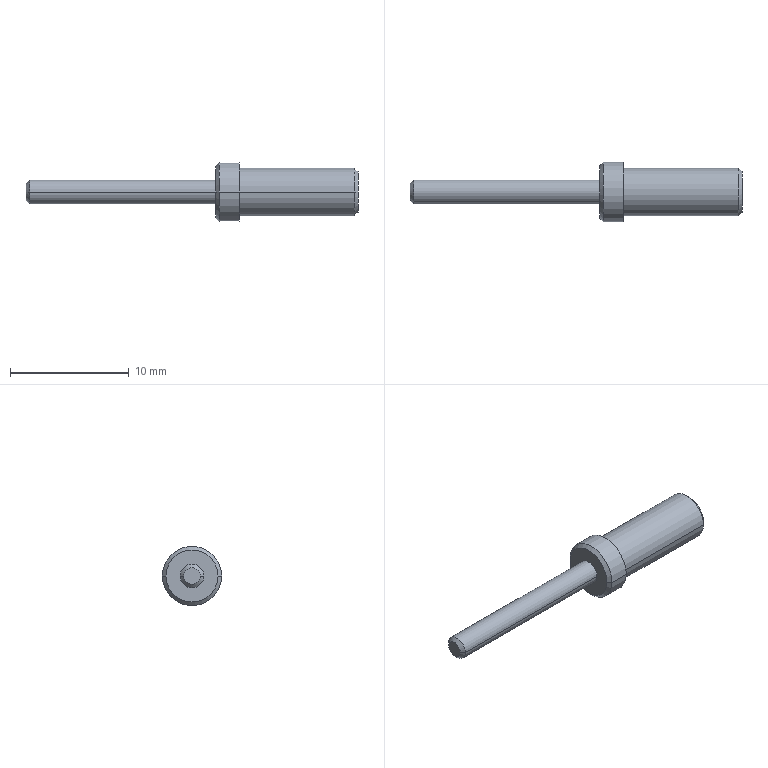Part | NX | 1 solid | 16 faces | box 28 x 5 x 5 mm | volume 213.729 mm3 | cylinder 6 | cone 6 | plane 4 | commonest cylinder face diameters 2 x2 4 x2 5 x2
STEP:
#1=CARTESIAN_POINT('',(2216.,157.,-96.));
#2=VERTEX_POINT('',#1);
#3=CARTESIAN_POINT('',(2216.,153.,-96.));
#4=VERTEX_POINT('',#3);
#5=CARTESIAN_POINT('',(2216.,155.,-96.));
#6=DIRECTION('',(1.,0.,0.));
#7=DIRECTION('',(0.,1.,0.));
#8=AXIS2_PLACEMENT_3D('',#5,#6,#7);
#9=CIRCLE('',#8,2.);
#10=EDGE_CURVE('',#2,#4,#9,.T.);
#11=ORIENTED_EDGE('',*,*,#10,.T.);
#12=CARTESIAN_POINT('',(2225.7,153.,-96.));
#13=VERTEX_POINT('',#12);
#14=CARTESIAN_POINT('',(2216.,153.,-96.));
#15=DIRECTION('',(1.,0.,0.));
#16=VECTOR('',#15,1000.);
#17=LINE('',#14,#16);
#18=EDGE_CURVE('',#4,#13,#17,.T.);
#19=ORIENTED_EDGE('',*,*,#18,.T.);
#20=CARTESIAN_POINT('',(2225.7,157.,-96.));
#21=VERTEX_POINT('',#20);
#22=CARTESIAN_POINT('',(2225.7,155.,-96.));
#23=DIRECTION('',(1.,0.,0.));
#24=DIRECTION('',(0.,1.,0.));
#25=AXIS2_PLACEMENT_3D('',#22,#23,#24);
#26=CIRCLE('',#25,2.);
#27=EDGE_CURVE('',#21,#13,#26,.T.);
#28=ORIENTED_EDGE('',*,*,#27,.F.);
#29=CARTESIAN_POINT('',(2216.,157.,-96.));
#30=DIRECTION('',(1.,0.,0.));
#31=VECTOR('',#30,1000.);
#32=LINE('',#29,#31);
#33=EDGE_CURVE('',#2,#21,#32,.T.);
#34=ORIENTED_EDGE('',*,*,#33,.F.);
#35=EDGE_LOOP('',(#11,#19,#28,#34));
#36=FACE_BOUND('',#35,.T.);
#37=CARTESIAN_POINT('',(2216.,155.,-96.));
#38=DIRECTION('',(1.,0.,0.));
#39=DIRECTION('',(0.,1.,0.));
#40=AXIS2_PLACEMENT_3D('',#37,#38,#39);
#41=CYLINDRICAL_SURFACE('',#40,2.);
#42=ADVANCED_FACE('',(#36),#41,.T.);
#43=CARTESIAN_POINT('',(2216.,152.5,-96.));
#44=VERTEX_POINT('',#43);
#45=CARTESIAN_POINT('',(2216.,157.5,-96.));
#46=VERTEX_POINT('',#45);
#47=CARTESIAN_POINT('',(2216.,155.,-96.));
#48=DIRECTION('',(1.,0.,0.));
#49=DIRECTION('',(0.,1.,0.));
#50=AXIS2_PLACEMENT_3D('',#47,#48,#49);
#51=CIRCLE('',#50,2.5);
#52=EDGE_CURVE('',#44,#46,#51,.T.);
#53=ORIENTED_EDGE('',*,*,#52,.T.);
#54=CARTESIAN_POINT('',(2216.,155.,-96.));
#55=DIRECTION('',(1.,0.,0.));
#56=DIRECTION('',(0.,1.,0.));
#57=AXIS2_PLACEMENT_3D('',#54,#55,#56);
#58=CIRCLE('',#57,2.5);
#59=EDGE_CURVE('',#46,#44,#58,.T.);
#60=ORIENTED_EDGE('',*,*,#59,.T.);
#61=EDGE_LOOP('',(#53,#60));
#62=FACE_BOUND('',#61,.T.);
#63=ORIENTED_EDGE('',*,*,#10,.F.);
#64=CARTESIAN_POINT('',(2216.,155.,-96.));
#65=DIRECTION('',(1.,0.,0.));
#66=DIRECTION('',(0.,1.,0.));
#67=AXIS2_PLACEMENT_3D('',#64,#65,#66);
#68=CIRCLE('',#67,2.);
#69=EDGE_CURVE('',#4,#2,#68,.T.);
#70=ORIENTED_EDGE('',*,*,#69,.F.);
#71=EDGE_LOOP('',(#63,#70));
#72=FACE_BOUND('',#71,.T.);
#73=CARTESIAN_POINT('',(2216.,153.76,-100.896));
#74=DIRECTION('',(1.,0.,0.));
#75=DIRECTION('',(0.,1.,0.));
#76=AXIS2_PLACEMENT_3D('',#73,#74,#75);
#77=PLANE('',#76);
#78=ADVANCED_FACE('',(#62,#72),#77,.T.);
#79=CARTESIAN_POINT('',(2214.3,152.5,-96.));
#80=VERTEX_POINT('',#79);
#81=CARTESIAN_POINT('',(2214.3,157.5,-96.));
#82=VERTEX_POINT('',#81);
#83=CARTESIAN_POINT('',(2214.3,155.,-96.));
#84=DIRECTION('',(1.,0.,0.));
#85=DIRECTION('',(0.,1.,0.));
#86=AXIS2_PLACEMENT_3D('',#83,#84,#85);
#87=CIRCLE('',#86,2.5);
#88=EDGE_CURVE('',#80,#82,#87,.T.);
#89=ORIENTED_EDGE('',*,*,#88,.T.);
#90=CARTESIAN_POINT('',(2216.,157.5,-96.));
#91=DIRECTION('',(1.,0.,0.));
#92=VECTOR('',#91,1000.);
#93=LINE('',#90,#92);
#94=EDGE_CURVE('',#82,#46,#93,.T.);
#95=ORIENTED_EDGE('',*,*,#94,.T.);
#96=ORIENTED_EDGE('',*,*,#52,.F.);
#97=CARTESIAN_POINT('',(2216.,152.5,-96.));
#98=DIRECTION('',(1.,0.,0.));
#99=VECTOR('',#98,1000.);
#100=LINE('',#97,#99);
#101=EDGE_CURVE('',#80,#44,#100,.T.);
#102=ORIENTED_EDGE('',*,*,#101,.F.);
#103=EDGE_LOOP('',(#89,#95,#96,#102));
#104=FACE_BOUND('',#103,.T.);
#105=CARTESIAN_POINT('',(2216.,155.,-96.));
#106=DIRECTION('',(1.,0.,0.));
#107=DIRECTION('',(0.,1.,0.));
#108=AXIS2_PLACEMENT_3D('',#105,#106,#107);
#109=CYLINDRICAL_SURFACE('',#108,2.5);
#110=ADVANCED_FACE('',(#104),#109,.T.);
#111=CARTESIAN_POINT('',(2214.,157.2,-96.));
#112=VERTEX_POINT('',#111);
#113=CARTESIAN_POINT('',(2214.,152.8,-96.));
#114=VERTEX_POINT('',#113);
#115=CARTESIAN_POINT('',(2214.,155.,-96.));
#116=DIRECTION('',(1.,0.,0.));
#117=DIRECTION('',(0.,1.,0.));
#118=AXIS2_PLACEMENT_3D('',#115,#116,#117);
#119=CIRCLE('',#118,2.2);
#120=EDGE_CURVE('',#112,#114,#119,.T.);
#121=ORIENTED_EDGE('',*,*,#120,.F.);
#122=CARTESIAN_POINT('',(2214.,155.,-96.));
#123=DIRECTION('',(1.,0.,0.));
#124=DIRECTION('',(0.,1.,0.));
#125=AXIS2_PLACEMENT_3D('',#122,#123,#124);
#126=CIRCLE('',#125,2.2);
#127=EDGE_CURVE('',#114,#112,#126,.T.);
#128=ORIENTED_EDGE('',*,*,#127,.F.);
#129=EDGE_LOOP('',(#121,#128));
#130=FACE_BOUND('',#129,.T.);
#131=CARTESIAN_POINT('',(2214.,156.,-96.));
#132=VERTEX_POINT('',#131);
#133=CARTESIAN_POINT('',(2214.,154.,-96.));
#134=VERTEX_POINT('',#133);
#135=CARTESIAN_POINT('',(2214.,155.,-96.));
#136=DIRECTION('',(-1.,0.,0.));
#137=DIRECTION('',(0.,-1.,0.));
#138=AXIS2_PLACEMENT_3D('',#135,#136,#137);
#139=CIRCLE('',#138,1.);
#140=EDGE_CURVE('',#132,#134,#139,.T.);
#141=ORIENTED_EDGE('',*,*,#140,.F.);
#142=CARTESIAN_POINT('',(2214.,155.,-96.));
#143=DIRECTION('',(-1.,0.,0.));
#144=DIRECTION('',(0.,-1.,0.));
#145=AXIS2_PLACEMENT_3D('',#142,#143,#144);
#146=CIRCLE('',#145,1.);
#147=EDGE_CURVE('',#134,#132,#146,.T.);
#148=ORIENTED_EDGE('',*,*,#147,.F.);
#149=EDGE_LOOP('',(#141,#148));
#150=FACE_BOUND('',#149,.T.);
#151=CARTESIAN_POINT('',(2214.,153.76,-100.896));
#152=DIRECTION('',(1.,0.,0.));
#153=DIRECTION('',(0.,1.,0.));
#154=AXIS2_PLACEMENT_3D('',#151,#152,#153);
#155=PLANE('',#154);
#156=ADVANCED_FACE('',(#130,#150),#155,.F.);
#157=CARTESIAN_POINT('',(2198.3,154.,-96.));
#158=VERTEX_POINT('',#157);
#159=CARTESIAN_POINT('',(2198.3,156.,-96.));
#160=VERTEX_POINT('',#159);
#161=CARTESIAN_POINT('',(2198.3,155.,-96.));
#162=DIRECTION('',(-1.,0.,0.));
#163=DIRECTION('',(0.,-1.,0.));
#164=AXIS2_PLACEMENT_3D('',#161,#162,#163);
#165=CIRCLE('',#164,1.);
#166=EDGE_CURVE('',#158,#160,#165,.T.);
#167=ORIENTED_EDGE('',*,*,#166,.F.);
#168=CARTESIAN_POINT('',(2214.,154.,-96.));
#169=DIRECTION('',(-1.,0.,0.));
#170=VECTOR('',#169,1000.);
#171=LINE('',#168,#170);
#172=EDGE_CURVE('',#158,#134,#171,.F.);
#173=ORIENTED_EDGE('',*,*,#172,.T.);
#174=ORIENTED_EDGE('',*,*,#147,.T.);
#175=CARTESIAN_POINT('',(2214.,156.,-96.));
#176=DIRECTION('',(-1.,0.,0.));
#177=VECTOR('',#176,1000.);
#178=LINE('',#175,#177);
#179=EDGE_CURVE('',#160,#132,#178,.F.);
#180=ORIENTED_EDGE('',*,*,#179,.F.);
#181=EDGE_LOOP('',(#167,#173,#174,#180));
#182=FACE_BOUND('',#181,.T.);
#183=CARTESIAN_POINT('',(2214.,155.,-96.));
#184=DIRECTION('',(-1.,0.,0.));
#185=DIRECTION('',(0.,-1.,0.));
#186=AXIS2_PLACEMENT_3D('',#183,#184,#185);
#187=CYLINDRICAL_SURFACE('',#186,1.);
#188=ADVANCED_FACE('',(#182),#187,.T.);
#189=CARTESIAN_POINT('',(2198.,155.7,-96.));
#190=VERTEX_POINT('',#189);
#191=CARTESIAN_POINT('',(2198.,154.3,-96.));
#192=VERTEX_POINT('',#191);
#193=CARTESIAN_POINT('',(2198.,155.,-96.));
#194=DIRECTION('',(-1.,0.,0.));
#195=DIRECTION('',(0.,-1.,0.));
#196=AXIS2_PLACEMENT_3D('',#193,#194,#195);
#197=CIRCLE('',#196,0.7);
#198=EDGE_CURVE('',#190,#192,#197,.T.);
#199=ORIENTED_EDGE('',*,*,#198,.T.);
#200=CARTESIAN_POINT('',(2198.,155.,-96.));
#201=DIRECTION('',(-1.,0.,0.));
#202=DIRECTION('',(0.,-1.,0.));
#203=AXIS2_PLACEMENT_3D('',#200,#201,#202);
#204=CIRCLE('',#203,0.7);
#205=EDGE_CURVE('',#192,#190,#204,.T.);
#206=ORIENTED_EDGE('',*,*,#205,.T.);
#207=EDGE_LOOP('',(#199,#206));
#208=FACE_BOUND('',#207,.T.);
#209=CARTESIAN_POINT('',(2198.,154.151,-95.92));
#210=DIRECTION('',(-1.,0.,0.));
#211=DIRECTION('',(0.,0.,1.));
#212=AXIS2_PLACEMENT_3D('',#209,#210,#211);
#213=PLANE('',#212);
#214=ADVANCED_FACE('',(#208),#213,.T.);
#215=ORIENTED_EDGE('',*,*,#120,.T.);
#216=CARTESIAN_POINT('',(2214.,152.8,-96.));
#217=DIRECTION('',(0.7071,-0.7071,0.));
#218=VECTOR('',#217,1000.);
#219=LINE('',#216,#218);
#220=EDGE_CURVE('',#80,#114,#219,.F.);
#221=ORIENTED_EDGE('',*,*,#220,.F.);
#222=CARTESIAN_POINT('',(2214.3,155.,-96.));
#223=DIRECTION('',(1.,0.,0.));
#224=DIRECTION('',(0.,1.,0.));
#225=AXIS2_PLACEMENT_3D('',#222,#223,#224);
#226=CIRCLE('',#225,2.5);
#227=EDGE_CURVE('',#82,#80,#226,.T.);
#228=ORIENTED_EDGE('',*,*,#227,.F.);
#229=CARTESIAN_POINT('',(2214.,157.2,-96.));
#230=DIRECTION('',(0.7071,0.7071,0.));
#231=VECTOR('',#230,1000.);
#232=LINE('',#229,#231);
#233=EDGE_CURVE('',#82,#112,#232,.F.);
#234=ORIENTED_EDGE('',*,*,#233,.T.);
#235=EDGE_LOOP('',(#215,#221,#228,#234));
#236=FACE_BOUND('',#235,.T.);
#237=CARTESIAN_POINT('',(2214.,155.,-96.));
#238=DIRECTION('',(1.,0.,0.));
#239=DIRECTION('',(0.,-1.,0.));
#240=AXIS2_PLACEMENT_3D('',#237,#238,#239);
#241=CONICAL_SURFACE('',#240,2.2,0.7854);
#242=ADVANCED_FACE('',(#236),#241,.T.);
#243=ORIENTED_EDGE('',*,*,#198,.F.);
#244=CARTESIAN_POINT('',(2198.,155.7,-96.));
#245=DIRECTION('',(0.7071,0.7071,0.));
#246=VECTOR('',#245,1000.);
#247=LINE('',#244,#246);
#248=EDGE_CURVE('',#190,#160,#247,.T.);
#249=ORIENTED_EDGE('',*,*,#248,.T.);
#250=CARTESIAN_POINT('',(2198.3,155.,-96.));
#251=DIRECTION('',(-1.,0.,0.));
#252=DIRECTION('',(0.,-1.,0.));
#253=AXIS2_PLACEMENT_3D('',#250,#251,#252);
#254=CIRCLE('',#253,1.);
#255=EDGE_CURVE('',#160,#158,#254,.T.);
#256=ORIENTED_EDGE('',*,*,#255,.T.);
#257=CARTESIAN_POINT('',(2198.,154.3,-96.));
#258=DIRECTION('',(0.7071,-0.7071,0.));
#259=VECTOR('',#258,1000.);
#260=LINE('',#257,#259);
#261=EDGE_CURVE('',#192,#158,#260,.T.);
#262=ORIENTED_EDGE('',*,*,#261,.F.);
#263=EDGE_LOOP('',(#243,#249,#256,#262));
#264=FACE_BOUND('',#263,.T.);
#265=CARTESIAN_POINT('',(2198.,155.,-96.));
#266=DIRECTION('',(1.,0.,0.));
#267=DIRECTION('',(0.,-1.,0.));
#268=AXIS2_PLACEMENT_3D('',#265,#266,#267);
#269=CONICAL_SURFACE('',#268,0.7,0.7854);
#270=ADVANCED_FACE('',(#264),#269,.T.);
#271=ORIENTED_EDGE('',*,*,#27,.T.);
#272=CARTESIAN_POINT('',(2226.,153.3,-96.));
#273=VERTEX_POINT('',#272);
#274=CARTESIAN_POINT('',(2226.,153.3,-96.));
#275=DIRECTION('',(-0.7071,-0.7071,0.));
#276=VECTOR('',#275,1000.);
#277=LINE('',#274,#276);
#278=EDGE_CURVE('',#13,#273,#277,.F.);
#279=ORIENTED_EDGE('',*,*,#278,.T.);
#280=CARTESIAN_POINT('',(2226.,156.7,-96.));
#281=VERTEX_POINT('',#280);
#282=CARTESIAN_POINT('',(2226.,155.,-96.));
#283=DIRECTION('',(1.,0.,0.));
#284=DIRECTION('',(0.,1.,0.));
#285=AXIS2_PLACEMENT_3D('',#282,#283,#284);
#286=CIRCLE('',#285,1.7);
#287=EDGE_CURVE('',#281,#273,#286,.T.);
#288=ORIENTED_EDGE('',*,*,#287,.F.);
#289=CARTESIAN_POINT('',(2226.,156.7,-96.));
#290=DIRECTION('',(-0.7071,0.7071,0.));
#291=VECTOR('',#290,1000.);
#292=LINE('',#289,#291);
#293=EDGE_CURVE('',#21,#281,#292,.F.);
#294=ORIENTED_EDGE('',*,*,#293,.F.);
#295=EDGE_LOOP('',(#271,#279,#288,#294));
#296=FACE_BOUND('',#295,.T.);
#297=CARTESIAN_POINT('',(2226.,155.,-96.));
#298=DIRECTION('',(-1.,0.,0.));
#299=DIRECTION('',(0.,1.,0.));
#300=AXIS2_PLACEMENT_3D('',#297,#298,#299);
#301=CONICAL_SURFACE('',#300,1.7,0.7854);
#302=ADVANCED_FACE('',(#296),#301,.T.);
#303=CARTESIAN_POINT('',(2226.,155.,-96.));
#304=DIRECTION('',(1.,0.,0.));
#305=DIRECTION('',(0.,1.,0.));
#306=AXIS2_PLACEMENT_3D('',#303,#304,#305);
#307=CIRCLE('',#306,1.7);
#308=EDGE_CURVE('',#273,#281,#307,.T.);
#309=ORIENTED_EDGE('',*,*,#308,.T.);
#310=ORIENTED_EDGE('',*,*,#287,.T.);
#311=EDGE_LOOP('',(#309,#310));
#312=FACE_BOUND('',#311,.T.);
#313=CARTESIAN_POINT('',(2226.,153.76,-100.896));
#314=DIRECTION('',(1.,0.,0.));
#315=DIRECTION('',(0.,1.,0.));
#316=AXIS2_PLACEMENT_3D('',#313,#314,#315);
#317=PLANE('',#316);
#318=ADVANCED_FACE('',(#312),#317,.T.);
#319=ORIENTED_EDGE('',*,*,#94,.F.);
#320=ORIENTED_EDGE('',*,*,#227,.T.);
#321=ORIENTED_EDGE('',*,*,#101,.T.);
#322=ORIENTED_EDGE('',*,*,#59,.F.);
#323=EDGE_LOOP('',(#319,#320,#321,#322));
#324=FACE_BOUND('',#323,.T.);
#325=CARTESIAN_POINT('',(2216.,155.,-96.));
#326=DIRECTION('',(1.,0.,0.));
#327=DIRECTION('',(0.,1.,0.));
#328=AXIS2_PLACEMENT_3D('',#325,#326,#327);
#329=CYLINDRICAL_SURFACE('',#328,2.5);
#330=ADVANCED_FACE('',(#324),#329,.T.);
#331=ORIENTED_EDGE('',*,*,#308,.F.);
#332=ORIENTED_EDGE('',*,*,#278,.F.);
#333=CARTESIAN_POINT('',(2225.7,155.,-96.));
#334=DIRECTION('',(1.,0.,0.));
#335=DIRECTION('',(0.,1.,0.));
#336=AXIS2_PLACEMENT_3D('',#333,#334,#335);
#337=CIRCLE('',#336,2.);
#338=EDGE_CURVE('',#13,#21,#337,.T.);
#339=ORIENTED_EDGE('',*,*,#338,.T.);
#340=ORIENTED_EDGE('',*,*,#293,.T.);
#341=EDGE_LOOP('',(#331,#332,#339,#340));
#342=FACE_BOUND('',#341,.T.);
#343=CARTESIAN_POINT('',(2226.,155.,-96.));
#344=DIRECTION('',(-1.,0.,0.));
#345=DIRECTION('',(0.,1.,0.));
#346=AXIS2_PLACEMENT_3D('',#343,#344,#345);
#347=CONICAL_SURFACE('',#346,1.7,0.7854);
#348=ADVANCED_FACE('',(#342),#347,.T.);
#349=ORIENTED_EDGE('',*,*,#33,.T.);
#350=ORIENTED_EDGE('',*,*,#338,.F.);
#351=ORIENTED_EDGE('',*,*,#18,.F.);
#352=ORIENTED_EDGE('',*,*,#69,.T.);
#353=EDGE_LOOP('',(#349,#350,#351,#352));
#354=FACE_BOUND('',#353,.T.);
#355=CARTESIAN_POINT('',(2216.,155.,-96.));
#356=DIRECTION('',(1.,0.,0.));
#357=DIRECTION('',(0.,1.,0.));
#358=AXIS2_PLACEMENT_3D('',#355,#356,#357);
#359=CYLINDRICAL_SURFACE('',#358,2.);
#360=ADVANCED_FACE('',(#354),#359,.T.);
#361=ORIENTED_EDGE('',*,*,#166,.T.);
#362=ORIENTED_EDGE('',*,*,#248,.F.);
#363=ORIENTED_EDGE('',*,*,#205,.F.);
#364=ORIENTED_EDGE('',*,*,#261,.T.);
#365=EDGE_LOOP('',(#361,#362,#363,#364));
#366=FACE_BOUND('',#365,.T.);
#367=CARTESIAN_POINT('',(2198.,155.,-96.));
#368=DIRECTION('',(1.,0.,0.));
#369=DIRECTION('',(0.,-1.,0.));
#370=AXIS2_PLACEMENT_3D('',#367,#368,#369);
#371=CONICAL_SURFACE('',#370,0.7,0.7854);
#372=ADVANCED_FACE('',(#366),#371,.T.);
#373=ORIENTED_EDGE('',*,*,#140,.T.);
#374=ORIENTED_EDGE('',*,*,#172,.F.);
#375=ORIENTED_EDGE('',*,*,#255,.F.);
#376=ORIENTED_EDGE('',*,*,#179,.T.);
#377=EDGE_LOOP('',(#373,#374,#375,#376));
#378=FACE_BOUND('',#377,.T.);
#379=CARTESIAN_POINT('',(2214.,155.,-96.));
#380=DIRECTION('',(-1.,0.,0.));
#381=DIRECTION('',(0.,-1.,0.));
#382=AXIS2_PLACEMENT_3D('',#379,#380,#381);
#383=CYLINDRICAL_SURFACE('',#382,1.);
#384=ADVANCED_FACE('',(#378),#383,.T.);
#385=ORIENTED_EDGE('',*,*,#88,.F.);
#386=ORIENTED_EDGE('',*,*,#220,.T.);
#387=ORIENTED_EDGE('',*,*,#127,.T.);
#388=ORIENTED_EDGE('',*,*,#233,.F.);
#389=EDGE_LOOP('',(#385,#386,#387,#388));
#390=FACE_BOUND('',#389,.T.);
#391=CARTESIAN_POINT('',(2214.,155.,-96.));
#392=DIRECTION('',(1.,0.,0.));
#393=DIRECTION('',(0.,-1.,0.));
#394=AXIS2_PLACEMENT_3D('',#391,#392,#393);
#395=CONICAL_SURFACE('',#394,2.2,0.7854);
#396=ADVANCED_FACE('',(#390),#395,.T.);
#397=CLOSED_SHELL('',(#42,#78,#110,#156,#188,#214,#242,#270,#302,#318,#330,#348,#360,#372,#384,#396));
#398=MANIFOLD_SOLID_BREP('',#397);
#399=(LENGTH_UNIT()NAMED_UNIT(*)SI_UNIT(.MILLI.,.METRE.));
#400=UNCERTAINTY_MEASURE_WITH_UNIT(LENGTH_MEASURE(0.00001),#399,'','');
#401=(NAMED_UNIT(*)PLANE_ANGLE_UNIT()SI_UNIT($,.RADIAN.));
#402=(NAMED_UNIT(*)SI_UNIT($,.STERADIAN.)SOLID_ANGLE_UNIT());
#403=(GEOMETRIC_REPRESENTATION_CONTEXT(3)GLOBAL_UNCERTAINTY_ASSIGNED_CONTEXT((#400))GLOBAL_UNIT_ASSIGNED_CONTEXT((#399,#401,#402))REPRESENTATION_CONTEXT('',''));
#404=ADVANCED_BREP_SHAPE_REPRESENTATION('',(#398),#403);